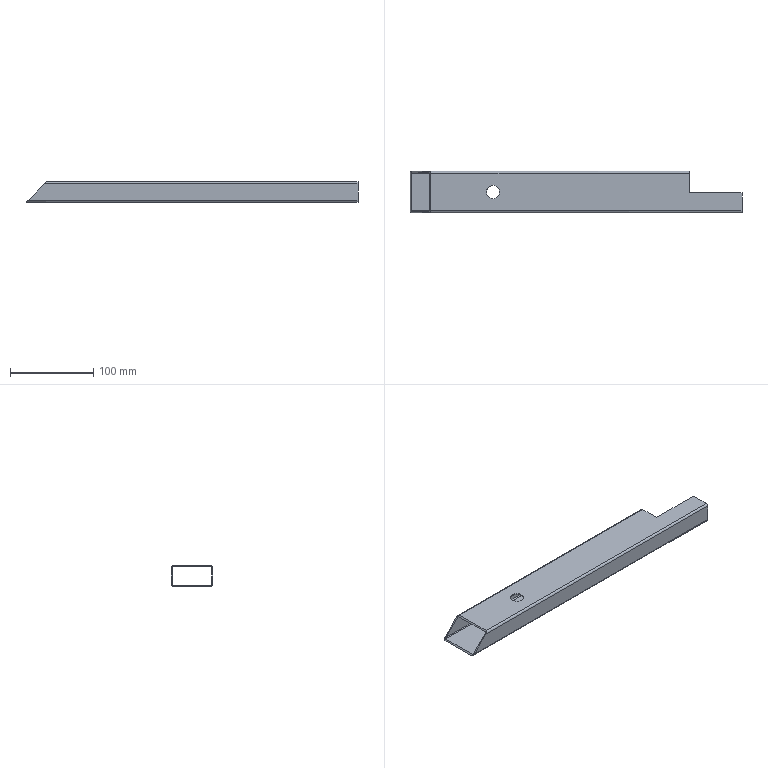Part | STEP file | 5090501R | 1 solid | 24 faces | box 400 x 50 x 25 mm | volume 74487 mm3 | plane 13 | cylinder 11 | commonest cylinder face diameters 2 x4 5 x4 16 x2 3.2 x1